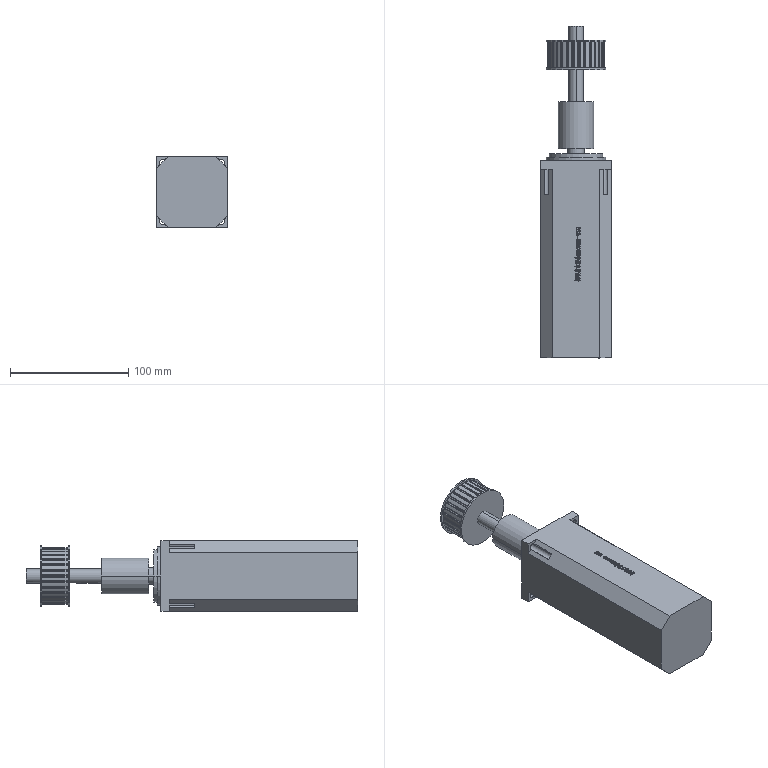Part | 4 solids | 1169 faces | box 60 x 280.8 x 60 mm | volume 655086 mm3 | plane 717 | spline 273 | cylinder 179 | commonest cylinder face diameters 0.96 x70 1.14 x40 47.75 x31 5.5 x8 4 x6 12 x6